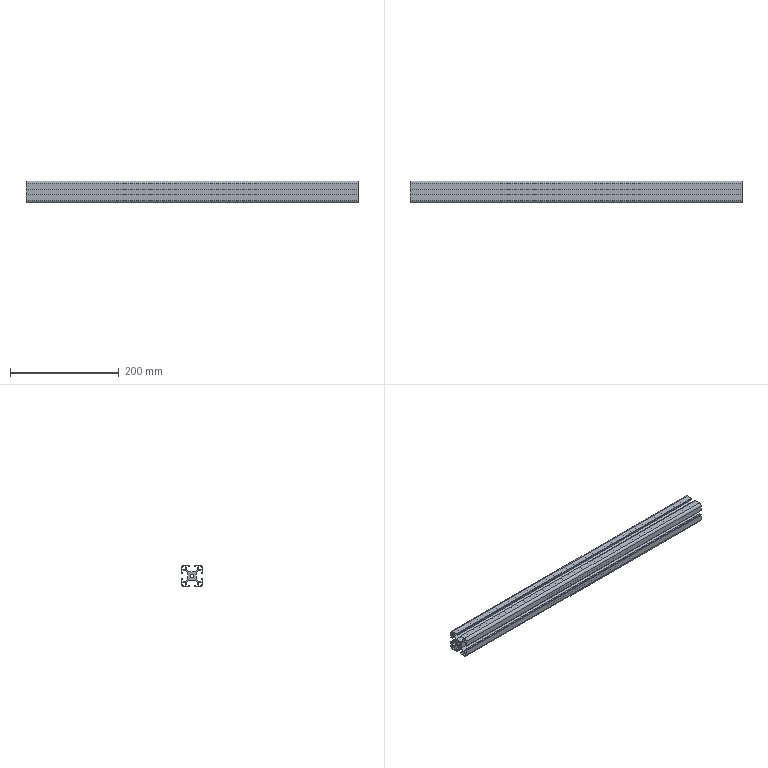Part | SolidWorks | features WeldMemberFeat 1, WeldmentFeature 1 | 1 solid | 104 faces | box 610 x 40 x 40 mm | volume 351693 mm3 | plane 94 | cylinder 10 | commonest cylinder face diameters 5 x4 9 x4 6.8 x2